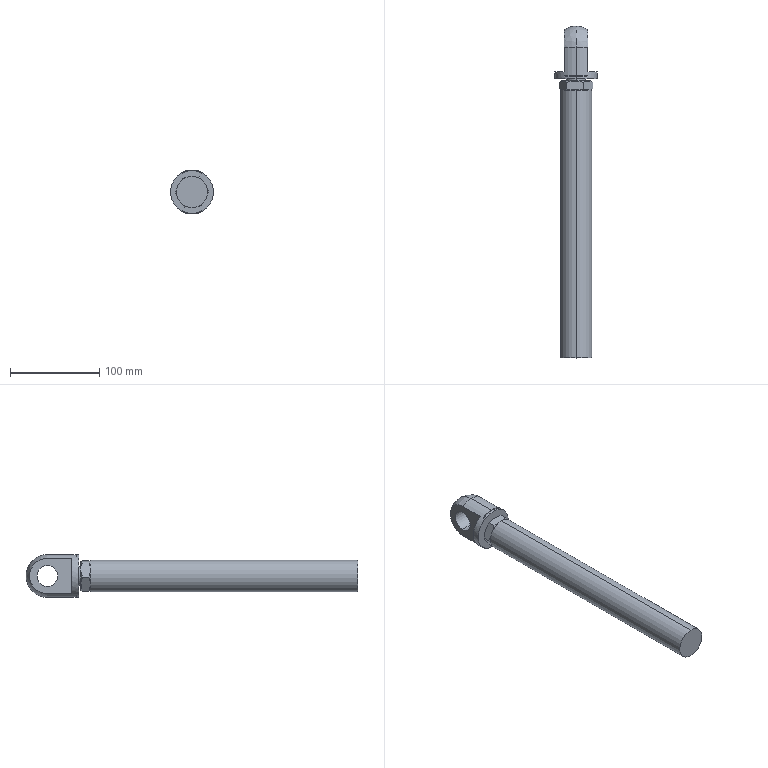Part | STEP file | Cylinder 2 | 3 solids | 46 faces | box 48 x 372 x 48.4 mm | volume 366109 mm3 | plane 22 | cylinder 14 | cone 8 | sphere 2 | commonest cylinder face diameters 20 x4 18.565 x2 21 x2 23.25 x2 35 x2 48 x2
STEP:
#1=CARTESIAN_POINT('',(-41.985,211.295,470.877));
#2=VERTEX_POINT('',#1);
#3=CARTESIAN_POINT('',(-40.938,211.901,470.948));
#4=VERTEX_POINT('',#3);
#5=CARTESIAN_POINT('',(-41.985,211.295,470.877));
#6=DIRECTION('',(0.864,0.5,0.05849));
#7=VECTOR('',#6,1000.);
#8=LINE('',#5,#7);
#9=EDGE_CURVE('',#2,#4,#8,.T.);
#10=ORIENTED_EDGE('',*,*,#9,.F.);
#11=CARTESIAN_POINT('',(-60.507,211.295,469.623));
#12=VERTEX_POINT('',#11);
#13=CARTESIAN_POINT('',(-51.246,211.295,470.25));
#14=DIRECTION('',(0.,1.,0.));
#15=DIRECTION('',(-0.9977,0.,-0.06754));
#16=AXIS2_PLACEMENT_3D('',#13,#14,#15);
#17=CIRCLE('',#16,9.282);
#18=EDGE_CURVE('',#12,#2,#17,.T.);
#19=ORIENTED_EDGE('',*,*,#18,.F.);
#20=CARTESIAN_POINT('',(-61.555,211.901,469.552));
#21=VERTEX_POINT('',#20);
#22=CARTESIAN_POINT('',(-60.507,211.295,469.623));
#23=DIRECTION('',(-0.864,0.5,-0.05849));
#24=VECTOR('',#23,1000.);
#25=LINE('',#22,#24);
#26=EDGE_CURVE('',#12,#21,#25,.T.);
#27=ORIENTED_EDGE('',*,*,#26,.T.);
#28=CARTESIAN_POINT('',(-51.246,211.901,470.25));
#29=DIRECTION('',(0.,-1.,0.));
#30=DIRECTION('',(-0.9977,0.,-0.06754));
#31=AXIS2_PLACEMENT_3D('',#28,#29,#30);
#32=CIRCLE('',#31,10.332);
#33=EDGE_CURVE('',#4,#21,#32,.T.);
#34=ORIENTED_EDGE('',*,*,#33,.F.);
#35=EDGE_LOOP('',(#10,#19,#27,#34));
#36=FACE_OUTER_BOUND('',#35,.T.);
#37=CARTESIAN_POINT('',(-51.246,211.295,470.25));
#38=DIRECTION('',(0.,1.,0.));
#39=DIRECTION('',(-0.9977,0.,-0.06754));
#40=AXIS2_PLACEMENT_3D('',#37,#38,#39);
#41=CONICAL_SURFACE('',#40,9.282,1.047);
#42=ADVANCED_FACE('',(#36),#41,.F.);
#43=CARTESIAN_POINT('',(-60.507,202.451,469.623));
#44=VERTEX_POINT('',#43);
#45=CARTESIAN_POINT('',(-61.112,201.401,469.582));
#46=VERTEX_POINT('',#45);
#47=CARTESIAN_POINT('',(-61.112,201.401,469.582));
#48=DIRECTION('',(-0.4989,-0.866,-0.03377));
#49=VECTOR('',#48,1000.);
#50=LINE('',#47,#49);
#51=EDGE_CURVE('',#44,#46,#50,.T.);
#52=ORIENTED_EDGE('',*,*,#51,.F.);
#53=CARTESIAN_POINT('',(-41.985,202.451,470.877));
#54=VERTEX_POINT('',#53);
#55=CARTESIAN_POINT('',(-51.246,202.451,470.25));
#56=DIRECTION('',(0.,-1.,0.));
#57=DIRECTION('',(-0.9977,0.,-0.06754));
#58=AXIS2_PLACEMENT_3D('',#55,#56,#57);
#59=CIRCLE('',#58,9.282);
#60=EDGE_CURVE('',#54,#44,#59,.T.);
#61=ORIENTED_EDGE('',*,*,#60,.F.);
#62=CARTESIAN_POINT('',(-41.381,201.401,470.918));
#63=VERTEX_POINT('',#62);
#64=CARTESIAN_POINT('',(-41.381,201.401,470.918));
#65=DIRECTION('',(0.4989,-0.866,0.03377));
#66=VECTOR('',#65,1000.);
#67=LINE('',#64,#66);
#68=EDGE_CURVE('',#54,#63,#67,.T.);
#69=ORIENTED_EDGE('',*,*,#68,.T.);
#70=CARTESIAN_POINT('',(-51.246,201.401,470.25));
#71=DIRECTION('',(0.,1.,0.));
#72=DIRECTION('',(-0.9977,0.,-0.06754));
#73=AXIS2_PLACEMENT_3D('',#70,#71,#72);
#74=CIRCLE('',#73,9.888);
#75=EDGE_CURVE('',#46,#63,#74,.T.);
#76=ORIENTED_EDGE('',*,*,#75,.F.);
#77=EDGE_LOOP('',(#52,#61,#69,#76));
#78=FACE_OUTER_BOUND('',#77,.T.);
#79=CARTESIAN_POINT('',(-51.246,201.401,470.25));
#80=DIRECTION('',(0.,-1.,0.));
#81=DIRECTION('',(0.9977,0.,0.06754));
#82=AXIS2_PLACEMENT_3D('',#79,#80,#81);
#83=CONICAL_SURFACE('',#82,9.888,0.5236);
#84=ADVANCED_FACE('',(#78),#83,.F.);
#85=CARTESIAN_POINT('',(-67.272,211.901,469.165));
#86=VERTEX_POINT('',#85);
#87=CARTESIAN_POINT('',(-69.967,210.341,468.983));
#88=VERTEX_POINT('',#87);
#89=CARTESIAN_POINT('',(-67.272,211.901,469.165));
#90=DIRECTION('',(-0.864,-0.5,-0.05849));
#91=VECTOR('',#90,1000.);
#92=LINE('',#89,#91);
#93=EDGE_CURVE('',#86,#88,#92,.T.);
#94=ORIENTED_EDGE('',*,*,#93,.F.);
#95=CARTESIAN_POINT('',(-35.221,211.901,471.335));
#96=VERTEX_POINT('',#95);
#97=CARTESIAN_POINT('',(-51.246,211.901,470.25));
#98=DIRECTION('',(0.,-1.,0.));
#99=DIRECTION('',(0.9977,0.,0.06754));
#100=AXIS2_PLACEMENT_3D('',#97,#98,#99);
#101=CIRCLE('',#100,16.063);
#102=EDGE_CURVE('',#86,#96,#101,.T.);
#103=ORIENTED_EDGE('',*,*,#102,.T.);
#104=CARTESIAN_POINT('',(-32.525,210.341,471.517));
#105=VERTEX_POINT('',#104);
#106=CARTESIAN_POINT('',(-35.221,211.901,471.335));
#107=DIRECTION('',(0.864,-0.5,0.05849));
#108=VECTOR('',#107,1000.);
#109=LINE('',#106,#108);
#110=EDGE_CURVE('',#96,#105,#109,.T.);
#111=ORIENTED_EDGE('',*,*,#110,.T.);
#112=CARTESIAN_POINT('',(-40.788,210.341,454.671));
#113=VERTEX_POINT('',#112);
#114=CARTESIAN_POINT('',(-32.525,210.341,471.517));
#115=CARTESIAN_POINT('',(-33.2,210.784,470.142));
#116=CARTESIAN_POINT('',(-33.879,211.148,468.757));
#117=CARTESIAN_POINT('',(-35.253,211.653,465.957));
#118=CARTESIAN_POINT('',(-35.946,211.792,464.542));
#119=CARTESIAN_POINT('',(-37.,211.793,462.394));
#120=CARTESIAN_POINT('',(-37.353,211.759,461.675));
#121=CARTESIAN_POINT('',(-38.051,211.627,460.251));
#122=CARTESIAN_POINT('',(-38.398,211.529,459.544));
#123=CARTESIAN_POINT('',(-39.432,211.15,457.436));
#124=CARTESIAN_POINT('',(-40.113,210.784,456.048));
#125=CARTESIAN_POINT('',(-40.788,210.341,454.671));
#126=B_SPLINE_CURVE_WITH_KNOTS('',3,(#114,#115,#116,#117,#118,#119,#120,#121,#122,#123,#124,#125),.UNSPECIFIED.,.F.,.F.,(4,2,2,2,2,4),(0.,0.004738,0.009475,0.01184,0.01421,0.01895),.UNSPECIFIED.);
#127=EDGE_CURVE('',#105,#113,#126,.T.);
#128=ORIENTED_EDGE('',*,*,#127,.T.);
#129=CARTESIAN_POINT('',(-59.509,210.341,453.403));
#130=VERTEX_POINT('',#129);
#131=CARTESIAN_POINT('',(-40.788,210.341,454.671));
#132=CARTESIAN_POINT('',(-42.317,210.784,454.567));
#133=CARTESIAN_POINT('',(-43.856,211.148,454.463));
#134=CARTESIAN_POINT('',(-46.967,211.653,454.252));
#135=CARTESIAN_POINT('',(-48.539,211.792,454.146));
#136=CARTESIAN_POINT('',(-50.927,211.793,453.984));
#137=CARTESIAN_POINT('',(-51.726,211.759,453.93));
#138=CARTESIAN_POINT('',(-53.308,211.627,453.823));
#139=CARTESIAN_POINT('',(-54.093,211.529,453.77));
#140=CARTESIAN_POINT('',(-56.436,211.15,453.612));
#141=CARTESIAN_POINT('',(-57.979,210.784,453.507));
#142=CARTESIAN_POINT('',(-59.509,210.341,453.403));
#143=B_SPLINE_CURVE_WITH_KNOTS('',3,(#131,#132,#133,#134,#135,#136,#137,#138,#139,#140,#141,#142),.UNSPECIFIED.,.F.,.F.,(4,2,2,2,2,4),(0.,0.004738,0.009475,0.01184,0.01421,0.01895),.UNSPECIFIED.);
#144=EDGE_CURVE('',#113,#130,#143,.T.);
#145=ORIENTED_EDGE('',*,*,#144,.T.);
#146=CARTESIAN_POINT('',(-59.509,210.341,453.403));
#147=CARTESIAN_POINT('',(-60.363,210.784,454.675));
#148=CARTESIAN_POINT('',(-61.223,211.148,455.957));
#149=CARTESIAN_POINT('',(-62.961,211.653,458.546));
#150=CARTESIAN_POINT('',(-63.839,211.792,459.854));
#151=CARTESIAN_POINT('',(-65.173,211.793,461.84));
#152=CARTESIAN_POINT('',(-65.62,211.759,462.506));
#153=CARTESIAN_POINT('',(-66.503,211.627,463.822));
#154=CARTESIAN_POINT('',(-66.942,211.529,464.476));
#155=CARTESIAN_POINT('',(-68.251,211.15,466.425));
#156=CARTESIAN_POINT('',(-69.113,210.784,467.709));
#157=CARTESIAN_POINT('',(-69.967,210.341,468.983));
#158=B_SPLINE_CURVE_WITH_KNOTS('',3,(#146,#147,#148,#149,#150,#151,#152,#153,#154,#155,#156,#157),.UNSPECIFIED.,.F.,.F.,(4,2,2,2,2,4),(0.,0.004738,0.009475,0.01184,0.01421,0.01895),.UNSPECIFIED.);
#159=EDGE_CURVE('',#130,#88,#158,.T.);
#160=ORIENTED_EDGE('',*,*,#159,.T.);
#161=EDGE_LOOP('',(#94,#103,#111,#128,#145,#160));
#162=FACE_OUTER_BOUND('',#161,.T.);
#163=CARTESIAN_POINT('',(-51.246,211.901,470.25));
#164=DIRECTION('',(0.,-1.,0.));
#165=DIRECTION('',(0.9977,0.,0.06754));
#166=AXIS2_PLACEMENT_3D('',#163,#164,#165);
#167=CONICAL_SURFACE('',#166,16.063,1.047);
#168=ADVANCED_FACE('',(#162),#167,.T.);
#169=CARTESIAN_POINT('',(-35.221,201.401,471.335));
#170=VERTEX_POINT('',#169);
#171=CARTESIAN_POINT('',(-32.525,202.961,471.517));
#172=VERTEX_POINT('',#171);
#173=CARTESIAN_POINT('',(-32.525,202.961,471.517));
#174=DIRECTION('',(0.864,0.5,0.05849));
#175=VECTOR('',#174,1000.);
#176=LINE('',#173,#175);
#177=EDGE_CURVE('',#170,#172,#176,.T.);
#178=ORIENTED_EDGE('',*,*,#177,.F.);
#179=CARTESIAN_POINT('',(-67.272,201.401,469.165));
#180=VERTEX_POINT('',#179);
#181=CARTESIAN_POINT('',(-51.246,201.401,470.25));
#182=DIRECTION('',(0.,-1.,0.));
#183=DIRECTION('',(0.9977,0.,0.06754));
#184=AXIS2_PLACEMENT_3D('',#181,#182,#183);
#185=CIRCLE('',#184,16.063);
#186=EDGE_CURVE('',#180,#170,#185,.T.);
#187=ORIENTED_EDGE('',*,*,#186,.F.);
#188=CARTESIAN_POINT('',(-69.967,202.961,468.983));
#189=VERTEX_POINT('',#188);
#190=CARTESIAN_POINT('',(-69.967,202.961,468.983));
#191=DIRECTION('',(-0.864,0.5,-0.05849));
#192=VECTOR('',#191,1000.);
#193=LINE('',#190,#192);
#194=EDGE_CURVE('',#180,#189,#193,.T.);
#195=ORIENTED_EDGE('',*,*,#194,.T.);
#196=CARTESIAN_POINT('',(-59.509,202.961,453.403));
#197=VERTEX_POINT('',#196);
#198=CARTESIAN_POINT('',(-69.967,202.961,468.983));
#199=CARTESIAN_POINT('',(-69.114,202.518,467.711));
#200=CARTESIAN_POINT('',(-68.254,202.154,466.43));
#201=CARTESIAN_POINT('',(-66.516,201.649,463.841));
#202=CARTESIAN_POINT('',(-65.638,201.51,462.532));
#203=CARTESIAN_POINT('',(-64.304,201.509,460.546));
#204=CARTESIAN_POINT('',(-63.857,201.543,459.88));
#205=CARTESIAN_POINT('',(-62.974,201.675,458.564));
#206=CARTESIAN_POINT('',(-62.535,201.773,457.91));
#207=CARTESIAN_POINT('',(-61.226,202.153,455.961));
#208=CARTESIAN_POINT('',(-60.364,202.518,454.677));
#209=CARTESIAN_POINT('',(-59.509,202.961,453.403));
#210=B_SPLINE_CURVE_WITH_KNOTS('',3,(#198,#199,#200,#201,#202,#203,#204,#205,#206,#207,#208,#209),.UNSPECIFIED.,.F.,.F.,(4,2,2,2,2,4),(0.,0.004738,0.009475,0.01184,0.01421,0.01895),.UNSPECIFIED.);
#211=EDGE_CURVE('',#189,#197,#210,.T.);
#212=ORIENTED_EDGE('',*,*,#211,.T.);
#213=CARTESIAN_POINT('',(-40.788,202.961,454.671));
#214=VERTEX_POINT('',#213);
#215=CARTESIAN_POINT('',(-59.509,202.961,453.403));
#216=CARTESIAN_POINT('',(-57.981,202.518,453.507));
#217=CARTESIAN_POINT('',(-56.441,202.154,453.611));
#218=CARTESIAN_POINT('',(-53.33,201.649,453.822));
#219=CARTESIAN_POINT('',(-51.758,201.51,453.928));
#220=CARTESIAN_POINT('',(-49.371,201.509,454.09));
#221=CARTESIAN_POINT('',(-48.571,201.543,454.144));
#222=CARTESIAN_POINT('',(-46.99,201.675,454.251));
#223=CARTESIAN_POINT('',(-46.204,201.773,454.304));
#224=CARTESIAN_POINT('',(-43.862,202.153,454.463));
#225=CARTESIAN_POINT('',(-42.319,202.518,454.567));
#226=CARTESIAN_POINT('',(-40.788,202.961,454.671));
#227=B_SPLINE_CURVE_WITH_KNOTS('',3,(#215,#216,#217,#218,#219,#220,#221,#222,#223,#224,#225,#226),.UNSPECIFIED.,.F.,.F.,(4,2,2,2,2,4),(0.,0.004738,0.009475,0.01184,0.01421,0.01895),.UNSPECIFIED.);
#228=EDGE_CURVE('',#197,#214,#227,.T.);
#229=ORIENTED_EDGE('',*,*,#228,.T.);
#230=CARTESIAN_POINT('',(-40.788,202.961,454.671));
#231=CARTESIAN_POINT('',(-40.114,202.518,456.046));
#232=CARTESIAN_POINT('',(-39.434,202.154,457.432));
#233=CARTESIAN_POINT('',(-38.061,201.649,460.231));
#234=CARTESIAN_POINT('',(-37.367,201.51,461.646));
#235=CARTESIAN_POINT('',(-36.314,201.509,463.794));
#236=CARTESIAN_POINT('',(-35.961,201.543,464.514));
#237=CARTESIAN_POINT('',(-35.263,201.675,465.937));
#238=CARTESIAN_POINT('',(-34.916,201.773,466.644));
#239=CARTESIAN_POINT('',(-33.882,202.153,468.752));
#240=CARTESIAN_POINT('',(-33.201,202.518,470.14));
#241=CARTESIAN_POINT('',(-32.525,202.961,471.517));
#242=B_SPLINE_CURVE_WITH_KNOTS('',3,(#230,#231,#232,#233,#234,#235,#236,#237,#238,#239,#240,#241),.UNSPECIFIED.,.F.,.F.,(4,2,2,2,2,4),(0.,0.004738,0.009475,0.01184,0.01421,0.01895),.UNSPECIFIED.);
#243=EDGE_CURVE('',#214,#172,#242,.T.);
#244=ORIENTED_EDGE('',*,*,#243,.T.);
#245=EDGE_LOOP('',(#178,#187,#195,#212,#229,#244));
#246=FACE_OUTER_BOUND('',#245,.T.);
#247=CARTESIAN_POINT('',(-51.246,202.961,470.25));
#248=DIRECTION('',(0.,1.,0.));
#249=DIRECTION('',(-0.9977,0.,-0.06754));
#250=AXIS2_PLACEMENT_3D('',#247,#248,#249);
#251=CONICAL_SURFACE('',#250,18.764,1.047);
#252=ADVANCED_FACE('',(#246),#251,.T.);
#253=CARTESIAN_POINT('',(-41.985,201.401,470.877));
#254=DIRECTION('',(0.,1.,0.));
#255=VECTOR('',#254,1000.);
#256=LINE('',#253,#255);
#257=EDGE_CURVE('',#54,#2,#256,.T.);
#258=ORIENTED_EDGE('',*,*,#257,.F.);
#259=ORIENTED_EDGE('',*,*,#60,.T.);
#260=CARTESIAN_POINT('',(-60.507,201.401,469.623));
#261=DIRECTION('',(0.,1.,0.));
#262=VECTOR('',#261,1000.);
#263=LINE('',#260,#262);
#264=EDGE_CURVE('',#44,#12,#263,.T.);
#265=ORIENTED_EDGE('',*,*,#264,.T.);
#266=ORIENTED_EDGE('',*,*,#18,.T.);
#267=EDGE_LOOP('',(#258,#259,#265,#266));
#268=FACE_OUTER_BOUND('',#267,.T.);
#269=CARTESIAN_POINT('',(-51.246,201.401,470.25));
#270=DIRECTION('',(0.,1.,0.));
#271=DIRECTION('',(-0.9977,0.,-0.06754));
#272=AXIS2_PLACEMENT_3D('',#269,#270,#271);
#273=CYLINDRICAL_SURFACE('',#272,9.282);
#274=ADVANCED_FACE('',(#268),#273,.F.);
#275=CARTESIAN_POINT('',(-51.246,211.901,470.25));
#276=DIRECTION('',(0.,-1.,0.));
#277=DIRECTION('',(-0.9977,0.,-0.06754));
#278=AXIS2_PLACEMENT_3D('',#275,#276,#277);
#279=CIRCLE('',#278,10.332);
#280=EDGE_CURVE('',#21,#4,#279,.T.);
#281=ORIENTED_EDGE('',*,*,#280,.T.);
#282=ORIENTED_EDGE('',*,*,#33,.T.);
#283=EDGE_LOOP('',(#281,#282));
#284=FACE_BOUND('',#283,.T.);
#285=CARTESIAN_POINT('',(-51.246,211.901,470.25));
#286=DIRECTION('',(0.,-1.,0.));
#287=DIRECTION('',(0.9977,0.,0.06754));
#288=AXIS2_PLACEMENT_3D('',#285,#286,#287);
#289=CIRCLE('',#288,16.063);
#290=EDGE_CURVE('',#96,#86,#289,.T.);
#291=ORIENTED_EDGE('',*,*,#290,.F.);
#292=ORIENTED_EDGE('',*,*,#102,.F.);
#293=EDGE_LOOP('',(#291,#292));
#294=FACE_OUTER_BOUND('',#293,.T.);
#295=CARTESIAN_POINT('',(-59.509,211.901,453.403));
#296=DIRECTION('',(0.,1.,0.));
#297=DIRECTION('',(-0.9977,0.,-0.06754));
#298=AXIS2_PLACEMENT_3D('',#295,#296,#297);
#299=PLANE('',#298);
#300=ADVANCED_FACE('',(#284,#294),#299,.T.);
#301=CARTESIAN_POINT('',(-51.246,201.401,470.25));
#302=DIRECTION('',(0.,1.,0.));
#303=DIRECTION('',(-0.9977,0.,-0.06754));
#304=AXIS2_PLACEMENT_3D('',#301,#302,#303);
#305=CIRCLE('',#304,9.888);
#306=EDGE_CURVE('',#63,#46,#305,.T.);
#307=ORIENTED_EDGE('',*,*,#306,.T.);
#308=ORIENTED_EDGE('',*,*,#75,.T.);
#309=EDGE_LOOP('',(#307,#308));
#310=FACE_BOUND('',#309,.T.);
#311=ORIENTED_EDGE('',*,*,#186,.T.);
#312=CARTESIAN_POINT('',(-51.246,201.401,470.25));
#313=DIRECTION('',(0.,-1.,0.));
#314=DIRECTION('',(0.9977,0.,0.06754));
#315=AXIS2_PLACEMENT_3D('',#312,#313,#314);
#316=CIRCLE('',#315,16.063);
#317=EDGE_CURVE('',#170,#180,#316,.T.);
#318=ORIENTED_EDGE('',*,*,#317,.T.);
#319=EDGE_LOOP('',(#311,#318));
#320=FACE_OUTER_BOUND('',#319,.T.);
#321=CARTESIAN_POINT('',(-59.509,201.401,453.403));
#322=DIRECTION('',(0.,1.,0.));
#323=DIRECTION('',(-0.9977,0.,-0.06754));
#324=AXIS2_PLACEMENT_3D('',#321,#322,#323);
#325=PLANE('',#324);
#326=ADVANCED_FACE('',(#310,#320),#325,.F.);
#327=ORIENTED_EDGE('',*,*,#159,.F.);
#328=CARTESIAN_POINT('',(-59.509,201.401,453.403));
#329=DIRECTION('',(0.,1.,0.));
#330=VECTOR('',#329,1000.);
#331=LINE('',#328,#330);
#332=EDGE_CURVE('',#197,#130,#331,.T.);
#333=ORIENTED_EDGE('',*,*,#332,.F.);
#334=ORIENTED_EDGE('',*,*,#211,.F.);
#335=CARTESIAN_POINT('',(-69.967,201.401,468.983));
#336=DIRECTION('',(0.,1.,0.));
#337=VECTOR('',#336,1000.);
#338=LINE('',#335,#337);
#339=EDGE_CURVE('',#189,#88,#338,.T.);
#340=ORIENTED_EDGE('',*,*,#339,.T.);
#341=EDGE_LOOP('',(#327,#333,#334,#340));
#342=FACE_OUTER_BOUND('',#341,.T.);
#343=CARTESIAN_POINT('',(-59.509,201.401,453.403));
#344=DIRECTION('',(-0.8303,0.,-0.5573));
#345=DIRECTION('',(0.,-1.,0.));
#346=AXIS2_PLACEMENT_3D('',#343,#344,#345);
#347=PLANE('',#346);
#348=ADVANCED_FACE('',(#342),#347,.T.);
#349=CARTESIAN_POINT('',(-61.704,210.341,485.829));
#350=VERTEX_POINT('',#349);
#351=CARTESIAN_POINT('',(-69.967,210.341,468.983));
#352=CARTESIAN_POINT('',(-69.293,210.784,470.358));
#353=CARTESIAN_POINT('',(-68.613,211.148,471.743));
#354=CARTESIAN_POINT('',(-67.24,211.653,474.543));
#355=CARTESIAN_POINT('',(-66.546,211.792,475.958));
#356=CARTESIAN_POINT('',(-65.493,211.793,478.106));
#357=CARTESIAN_POINT('',(-65.14,211.759,478.825));
#358=CARTESIAN_POINT('',(-64.442,211.627,480.249));
#359=CARTESIAN_POINT('',(-64.095,211.529,480.956));
#360=CARTESIAN_POINT('',(-63.061,211.15,483.064));
#361=CARTESIAN_POINT('',(-62.38,210.784,484.452));
#362=CARTESIAN_POINT('',(-61.704,210.341,485.829));
#363=B_SPLINE_CURVE_WITH_KNOTS('',3,(#351,#352,#353,#354,#355,#356,#357,#358,#359,#360,#361,#362),.UNSPECIFIED.,.F.,.F.,(4,2,2,2,2,4),(0.,0.004738,0.009475,0.01184,0.01421,0.01895),.UNSPECIFIED.);
#364=EDGE_CURVE('',#88,#350,#363,.T.);
#365=ORIENTED_EDGE('',*,*,#364,.F.);
#366=ORIENTED_EDGE('',*,*,#339,.F.);
#367=CARTESIAN_POINT('',(-61.704,202.961,485.829));
#368=VERTEX_POINT('',#367);
#369=CARTESIAN_POINT('',(-61.704,202.961,485.829));
#370=CARTESIAN_POINT('',(-62.379,202.518,484.454));
#371=CARTESIAN_POINT('',(-63.059,202.154,483.068));
#372=CARTESIAN_POINT('',(-64.432,201.649,480.269));
#373=CARTESIAN_POINT('',(-65.126,201.51,478.854));
#374=CARTESIAN_POINT('',(-66.179,201.509,476.706));
#375=CARTESIAN_POINT('',(-66.532,201.543,475.986));
#376=CARTESIAN_POINT('',(-67.23,201.675,474.563));
#377=CARTESIAN_POINT('',(-67.577,201.773,473.856));
#378=CARTESIAN_POINT('',(-68.611,202.153,471.748));
#379=CARTESIAN_POINT('',(-69.292,202.518,470.36));
#380=CARTESIAN_POINT('',(-69.967,202.961,468.983));
#381=B_SPLINE_CURVE_WITH_KNOTS('',3,(#369,#370,#371,#372,#373,#374,#375,#376,#377,#378,#379,#380),.UNSPECIFIED.,.F.,.F.,(4,2,2,2,2,4),(0.,0.004738,0.009475,0.01184,0.01421,0.01895),.UNSPECIFIED.);
#382=EDGE_CURVE('',#368,#189,#381,.T.);
#383=ORIENTED_EDGE('',*,*,#382,.F.);
#384=CARTESIAN_POINT('',(-61.704,201.401,485.829));
#385=DIRECTION('',(0.,1.,0.));
#386=VECTOR('',#385,1000.);
#387=LINE('',#384,#386);
#388=EDGE_CURVE('',#368,#350,#387,.T.);
#389=ORIENTED_EDGE('',*,*,#388,.T.);
#390=EDGE_LOOP('',(#365,#366,#383,#389));
#391=FACE_OUTER_BOUND('',#390,.T.);
#392=CARTESIAN_POINT('',(-69.967,201.401,468.983));
#393=DIRECTION('',(-0.8978,0.,0.4404));
#394=DIRECTION('',(0.,-1.,0.));
#395=AXIS2_PLACEMENT_3D('',#392,#393,#394);
#396=PLANE('',#395);
#397=ADVANCED_FACE('',(#391),#396,.T.);
#398=CARTESIAN_POINT('',(-42.983,210.341,487.097));
#399=VERTEX_POINT('',#398);
#400=CARTESIAN_POINT('',(-61.704,210.341,485.829));
#401=CARTESIAN_POINT('',(-60.176,210.784,485.933));
#402=CARTESIAN_POINT('',(-58.637,211.148,486.037));
#403=CARTESIAN_POINT('',(-55.525,211.653,486.248));
#404=CARTESIAN_POINT('',(-53.953,211.792,486.354));
#405=CARTESIAN_POINT('',(-51.566,211.793,486.516));
#406=CARTESIAN_POINT('',(-50.766,211.759,486.57));
#407=CARTESIAN_POINT('',(-49.185,211.627,486.677));
#408=CARTESIAN_POINT('',(-48.399,211.529,486.73));
#409=CARTESIAN_POINT('',(-46.057,211.15,486.888));
#410=CARTESIAN_POINT('',(-44.514,210.784,486.993));
#411=CARTESIAN_POINT('',(-42.983,210.341,487.097));
#412=B_SPLINE_CURVE_WITH_KNOTS('',3,(#400,#401,#402,#403,#404,#405,#406,#407,#408,#409,#410,#411),.UNSPECIFIED.,.F.,.F.,(4,2,2,2,2,4),(0.,0.004738,0.009475,0.01184,0.01421,0.01895),.UNSPECIFIED.);
#413=EDGE_CURVE('',#350,#399,#412,.T.);
#414=ORIENTED_EDGE('',*,*,#413,.F.);
#415=ORIENTED_EDGE('',*,*,#388,.F.);
#416=CARTESIAN_POINT('',(-42.983,202.961,487.097));
#417=VERTEX_POINT('',#416);
#418=CARTESIAN_POINT('',(-42.983,202.961,487.097));
#419=CARTESIAN_POINT('',(-44.512,202.518,486.993));
#420=CARTESIAN_POINT('',(-46.051,202.154,486.889));
#421=CARTESIAN_POINT('',(-49.163,201.649,486.678));
#422=CARTESIAN_POINT('',(-50.734,201.51,486.572));
#423=CARTESIAN_POINT('',(-53.122,201.509,486.41));
#424=CARTESIAN_POINT('',(-53.921,201.543,486.356));
#425=CARTESIAN_POINT('',(-55.503,201.675,486.249));
#426=CARTESIAN_POINT('',(-56.289,201.773,486.196));
#427=CARTESIAN_POINT('',(-58.631,202.153,486.037));
#428=CARTESIAN_POINT('',(-60.174,202.518,485.933));
#429=CARTESIAN_POINT('',(-61.704,202.961,485.829));
#430=B_SPLINE_CURVE_WITH_KNOTS('',3,(#418,#419,#420,#421,#422,#423,#424,#425,#426,#427,#428,#429),.UNSPECIFIED.,.F.,.F.,(4,2,2,2,2,4),(0.,0.004738,0.009475,0.01184,0.01421,0.01895),.UNSPECIFIED.);
#431=EDGE_CURVE('',#417,#368,#430,.T.);
#432=ORIENTED_EDGE('',*,*,#431,.F.);
#433=CARTESIAN_POINT('',(-42.983,201.401,487.097));
#434=DIRECTION('',(0.,1.,0.));
#435=VECTOR('',#434,1000.);
#436=LINE('',#433,#435);
#437=EDGE_CURVE('',#417,#399,#436,.T.);
#438=ORIENTED_EDGE('',*,*,#437,.T.);
#439=EDGE_LOOP('',(#414,#415,#432,#438));
#440=FACE_OUTER_BOUND('',#439,.T.);
#441=CARTESIAN_POINT('',(-61.704,201.401,485.829));
#442=DIRECTION('',(-0.06754,0.,0.9977));
#443=DIRECTION('',(-0.9977,0.,-0.06754));
#444=AXIS2_PLACEMENT_3D('',#441,#442,#443);
#445=PLANE('',#444);
#446=ADVANCED_FACE('',(#440),#445,.T.);
#447=CARTESIAN_POINT('',(-42.983,210.341,487.097));
#448=CARTESIAN_POINT('',(-42.13,210.784,485.825));
#449=CARTESIAN_POINT('',(-41.27,211.148,484.543));
#450=CARTESIAN_POINT('',(-39.532,211.653,481.954));
#451=CARTESIAN_POINT('',(-38.654,211.792,480.646));
#452=CARTESIAN_POINT('',(-37.32,211.793,478.66));
#453=CARTESIAN_POINT('',(-36.873,211.759,477.994));
#454=CARTESIAN_POINT('',(-35.99,211.627,476.678));
#455=CARTESIAN_POINT('',(-35.551,211.529,476.024));
#456=CARTESIAN_POINT('',(-34.242,211.15,474.075));
#457=CARTESIAN_POINT('',(-33.38,210.784,472.791));
#458=CARTESIAN_POINT('',(-32.525,210.341,471.517));
#459=B_SPLINE_CURVE_WITH_KNOTS('',3,(#447,#448,#449,#450,#451,#452,#453,#454,#455,#456,#457,#458),.UNSPECIFIED.,.F.,.F.,(4,2,2,2,2,4),(0.,0.004738,0.009475,0.01184,0.01421,0.01895),.UNSPECIFIED.);
#460=EDGE_CURVE('',#399,#105,#459,.T.);
#461=ORIENTED_EDGE('',*,*,#460,.F.);
#462=ORIENTED_EDGE('',*,*,#437,.F.);
#463=CARTESIAN_POINT('',(-32.525,202.961,471.517));
#464=CARTESIAN_POINT('',(-33.379,202.518,472.789));
#465=CARTESIAN_POINT('',(-34.239,202.154,474.07));
#466=CARTESIAN_POINT('',(-35.977,201.649,476.659));
#467=CARTESIAN_POINT('',(-36.855,201.51,477.968));
#468=CARTESIAN_POINT('',(-38.189,201.509,479.954));
#469=CARTESIAN_POINT('',(-38.636,201.543,480.62));
#470=CARTESIAN_POINT('',(-39.519,201.675,481.936));
#471=CARTESIAN_POINT('',(-39.958,201.773,482.59));
#472=CARTESIAN_POINT('',(-41.267,202.153,484.539));
#473=CARTESIAN_POINT('',(-42.129,202.518,485.823));
#474=CARTESIAN_POINT('',(-42.983,202.961,487.097));
#475=B_SPLINE_CURVE_WITH_KNOTS('',3,(#463,#464,#465,#466,#467,#468,#469,#470,#471,#472,#473,#474),.UNSPECIFIED.,.F.,.F.,(4,2,2,2,2,4),(0.,0.004738,0.009475,0.01184,0.01421,0.01895),.UNSPECIFIED.);
#476=EDGE_CURVE('',#172,#417,#475,.T.);
#477=ORIENTED_EDGE('',*,*,#476,.F.);
#478=CARTESIAN_POINT('',(-32.525,201.401,471.517));
#479=DIRECTION('',(0.,1.,0.));
#480=VECTOR('',#479,1000.);
#481=LINE('',#478,#480);
#482=EDGE_CURVE('',#172,#105,#481,.T.);
#483=ORIENTED_EDGE('',*,*,#482,.T.);
#484=EDGE_LOOP('',(#461,#462,#477,#483));
#485=FACE_OUTER_BOUND('',#484,.T.);
#486=CARTESIAN_POINT('',(-42.983,201.401,487.097));
#487=DIRECTION('',(0.8303,0.,0.5573));
#488=DIRECTION('',(0.,1.,0.));
#489=AXIS2_PLACEMENT_3D('',#486,#487,#488);
#490=PLANE('',#489);
#491=ADVANCED_FACE('',(#485),#490,.T.);
#492=ORIENTED_EDGE('',*,*,#127,.F.);
#493=ORIENTED_EDGE('',*,*,#482,.F.);
#494=ORIENTED_EDGE('',*,*,#243,.F.);
#495=CARTESIAN_POINT('',(-40.788,201.401,454.671));
#496=DIRECTION('',(0.,1.,0.));
#497=VECTOR('',#496,1000.);
#498=LINE('',#495,#497);
#499=EDGE_CURVE('',#214,#113,#498,.T.);
#500=ORIENTED_EDGE('',*,*,#499,.T.);
#501=EDGE_LOOP('',(#492,#493,#494,#500));
#502=FACE_OUTER_BOUND('',#501,.T.);
#503=CARTESIAN_POINT('',(-32.525,201.401,471.517));
#504=DIRECTION('',(0.8978,0.,-0.4404));
#505=DIRECTION('',(0.4404,0.,0.8978));
#506=AXIS2_PLACEMENT_3D('',#503,#504,#505);
#507=PLANE('',#506);
#508=ADVANCED_FACE('',(#502),#507,.T.);
#509=ORIENTED_EDGE('',*,*,#144,.F.);
#510=ORIENTED_EDGE('',*,*,#499,.F.);
#511=ORIENTED_EDGE('',*,*,#228,.F.);
#512=ORIENTED_EDGE('',*,*,#332,.T.);
#513=EDGE_LOOP('',(#509,#510,#511,#512));
#514=FACE_OUTER_BOUND('',#513,.T.);
#515=CARTESIAN_POINT('',(-40.788,201.401,454.671));
#516=DIRECTION('',(0.06754,0.,-0.9977));
#517=DIRECTION('',(0.,-1.,0.));
#518=AXIS2_PLACEMENT_3D('',#515,#516,#517);
#519=PLANE('',#518);
#520=ADVANCED_FACE('',(#514),#519,.T.);
#521=CARTESIAN_POINT('',(-51.246,202.451,470.25));
#522=DIRECTION('',(0.,-1.,0.));
#523=DIRECTION('',(-0.9977,0.,-0.06754));
#524=AXIS2_PLACEMENT_3D('',#521,#522,#523);
#525=CIRCLE('',#524,9.282);
#526=EDGE_CURVE('',#44,#54,#525,.T.);
#527=ORIENTED_EDGE('',*,*,#526,.T.);
#528=ORIENTED_EDGE('',*,*,#257,.T.);
#529=CARTESIAN_POINT('',(-51.246,211.295,470.25));
#530=DIRECTION('',(0.,1.,0.));
#531=DIRECTION('',(-0.9977,0.,-0.06754));
#532=AXIS2_PLACEMENT_3D('',#529,#530,#531);
#533=CIRCLE('',#532,9.282);
#534=EDGE_CURVE('',#2,#12,#533,.T.);
#535=ORIENTED_EDGE('',*,*,#534,.T.);
#536=ORIENTED_EDGE('',*,*,#264,.F.);
#537=EDGE_LOOP('',(#527,#528,#535,#536));
#538=FACE_OUTER_BOUND('',#537,.T.);
#539=CARTESIAN_POINT('',(-51.246,201.401,470.25));
#540=DIRECTION('',(0.,1.,0.));
#541=DIRECTION('',(-0.9977,0.,-0.06754));
#542=AXIS2_PLACEMENT_3D('',#539,#540,#541);
#543=CYLINDRICAL_SURFACE('',#542,9.282);
#544=ADVANCED_FACE('',(#538),#543,.F.);
#545=ORIENTED_EDGE('',*,*,#317,.F.);
#546=ORIENTED_EDGE('',*,*,#177,.T.);
#547=ORIENTED_EDGE('',*,*,#476,.T.);
#548=ORIENTED_EDGE('',*,*,#431,.T.);
#549=ORIENTED_EDGE('',*,*,#382,.T.);
#550=ORIENTED_EDGE('',*,*,#194,.F.);
#551=EDGE_LOOP('',(#545,#546,#547,#548,#549,#550));
#552=FACE_OUTER_BOUND('',#551,.T.);
#553=CARTESIAN_POINT('',(-51.246,202.961,470.25));
#554=DIRECTION('',(0.,1.,0.));
#555=DIRECTION('',(-0.9977,0.,-0.06754));
#556=AXIS2_PLACEMENT_3D('',#553,#554,#555);
#557=CONICAL_SURFACE('',#556,18.764,1.047);
#558=ADVANCED_FACE('',(#552),#557,.T.);
#559=ORIENTED_EDGE('',*,*,#290,.T.);
#560=ORIENTED_EDGE('',*,*,#93,.T.);
#561=ORIENTED_EDGE('',*,*,#364,.T.);
#562=ORIENTED_EDGE('',*,*,#413,.T.);
#563=ORIENTED_EDGE('',*,*,#460,.T.);
#564=ORIENTED_EDGE('',*,*,#110,.F.);
#565=EDGE_LOOP('',(#559,#560,#561,#562,#563,#564));
#566=FACE_OUTER_BOUND('',#565,.T.);
#567=CARTESIAN_POINT('',(-51.246,211.901,470.25));
#568=DIRECTION('',(0.,-1.,0.));
#569=DIRECTION('',(0.9977,0.,0.06754));
#570=AXIS2_PLACEMENT_3D('',#567,#568,#569);
#571=CONICAL_SURFACE('',#570,16.063,1.047);
#572=ADVANCED_FACE('',(#566),#571,.T.);
#573=ORIENTED_EDGE('',*,*,#526,.F.);
#574=ORIENTED_EDGE('',*,*,#51,.T.);
#575=ORIENTED_EDGE('',*,*,#306,.F.);
#576=ORIENTED_EDGE('',*,*,#68,.F.);
#577=EDGE_LOOP('',(#573,#574,#575,#576));
#578=FACE_OUTER_BOUND('',#577,.T.);
#579=CARTESIAN_POINT('',(-51.246,201.401,470.25));
#580=DIRECTION('',(0.,-1.,0.));
#581=DIRECTION('',(0.9977,0.,0.06754));
#582=AXIS2_PLACEMENT_3D('',#579,#580,#581);
#583=CONICAL_SURFACE('',#582,9.888,0.5236);
#584=ADVANCED_FACE('',(#578),#583,.F.);
#585=ORIENTED_EDGE('',*,*,#534,.F.);
#586=ORIENTED_EDGE('',*,*,#9,.T.);
#587=ORIENTED_EDGE('',*,*,#280,.F.);
#588=ORIENTED_EDGE('',*,*,#26,.F.);
#589=EDGE_LOOP('',(#585,#586,#587,#588));
#590=FACE_OUTER_BOUND('',#589,.T.);
#591=CARTESIAN_POINT('',(-51.246,211.295,470.25));
#592=DIRECTION('',(0.,1.,0.));
#593=DIRECTION('',(-0.9977,0.,-0.06754));
#594=AXIS2_PLACEMENT_3D('',#591,#592,#593);
#595=CONICAL_SURFACE('',#594,9.282,1.047);
#596=ADVANCED_FACE('',(#590),#595,.F.);
#597=CLOSED_SHELL('',(#42,#84,#168,#252,#274,#300,#326,#348,#397,#446,#491,#508,#520,#544,#558,#572,#584,#596));
#598=MANIFOLD_SOLID_BREP('',#597);
#599=CARTESIAN_POINT('',(-51.246,-98.599,452.75));
#600=VERTEX_POINT('',#599);
#601=CARTESIAN_POINT('',(-51.246,-98.599,487.75));
#602=VERTEX_POINT('',#601);
#603=CARTESIAN_POINT('',(-51.246,-98.599,470.25));
#604=DIRECTION('',(0.,1.,0.));
#605=DIRECTION('',(0.,0.,1.));
#606=AXIS2_PLACEMENT_3D('',#603,#604,#605);
#607=CIRCLE('',#606,17.5);
#608=EDGE_CURVE('',#600,#602,#607,.T.);
#609=ORIENTED_EDGE('',*,*,#608,.F.);
#610=CARTESIAN_POINT('',(-51.246,-98.599,470.25));
#611=DIRECTION('',(0.,1.,0.));
#612=DIRECTION('',(0.,0.,1.));
#613=AXIS2_PLACEMENT_3D('',#610,#611,#612);
#614=CIRCLE('',#613,17.5);
#615=EDGE_CURVE('',#602,#600,#614,.T.);
#616=ORIENTED_EDGE('',*,*,#615,.F.);
#617=EDGE_LOOP('',(#609,#616));
#618=FACE_OUTER_BOUND('',#617,.T.);
#619=CARTESIAN_POINT('',(-51.246,-98.599,470.25));
#620=DIRECTION('',(0.,1.,0.));
#621=DIRECTION('',(1.,0.,0.));
#622=AXIS2_PLACEMENT_3D('',#619,#620,#621);
#623=PLANE('',#622);
#624=ADVANCED_FACE('',(#618),#623,.F.);
#625=CARTESIAN_POINT('',(-51.246,201.401,452.75));
#626=VERTEX_POINT('',#625);
#627=CARTESIAN_POINT('',(-51.246,201.401,487.75));
#628=VERTEX_POINT('',#627);
#629=CARTESIAN_POINT('',(-51.246,201.401,470.25));
#630=DIRECTION('',(0.,1.,0.));
#631=DIRECTION('',(0.,0.,1.));
#632=AXIS2_PLACEMENT_3D('',#629,#630,#631);
#633=CIRCLE('',#632,17.5);
#634=EDGE_CURVE('',#626,#628,#633,.T.);
#635=ORIENTED_EDGE('',*,*,#634,.T.);
#636=CARTESIAN_POINT('',(-51.246,201.401,470.25));
#637=DIRECTION('',(0.,1.,0.));
#638=DIRECTION('',(0.,0.,1.));
#639=AXIS2_PLACEMENT_3D('',#636,#637,#638);
#640=CIRCLE('',#639,17.5);
#641=EDGE_CURVE('',#628,#626,#640,.T.);
#642=ORIENTED_EDGE('',*,*,#641,.T.);
#643=EDGE_LOOP('',(#635,#642));
#644=FACE_OUTER_BOUND('',#643,.T.);
#645=CARTESIAN_POINT('',(-51.246,201.401,470.25));
#646=DIRECTION('',(0.,1.,0.));
#647=DIRECTION('',(1.,0.,0.));
#648=AXIS2_PLACEMENT_3D('',#645,#646,#647);
#649=PLANE('',#648);
#650=ADVANCED_FACE('',(#644),#649,.T.);
#651=CARTESIAN_POINT('',(-51.246,201.401,487.75));
#652=DIRECTION('',(0.,-1.,0.));
#653=VECTOR('',#652,1000.);
#654=LINE('',#651,#653);
#655=EDGE_CURVE('',#628,#602,#654,.T.);
#656=ORIENTED_EDGE('',*,*,#655,.F.);
#657=ORIENTED_EDGE('',*,*,#634,.F.);
#658=CARTESIAN_POINT('',(-51.246,201.401,452.75));
#659=DIRECTION('',(0.,-1.,0.));
#660=VECTOR('',#659,1000.);
#661=LINE('',#658,#660);
#662=EDGE_CURVE('',#626,#600,#661,.T.);
#663=ORIENTED_EDGE('',*,*,#662,.T.);
#664=ORIENTED_EDGE('',*,*,#608,.T.);
#665=EDGE_LOOP('',(#656,#657,#663,#664));
#666=FACE_OUTER_BOUND('',#665,.T.);
#667=CARTESIAN_POINT('',(-51.246,201.401,470.25));
#668=DIRECTION('',(0.,-1.,0.));
#669=DIRECTION('',(0.,0.,-1.));
#670=AXIS2_PLACEMENT_3D('',#667,#668,#669);
#671=CYLINDRICAL_SURFACE('',#670,17.5);
#672=ADVANCED_FACE('',(#666),#671,.T.);
#673=ORIENTED_EDGE('',*,*,#641,.F.);
#674=ORIENTED_EDGE('',*,*,#655,.T.);
#675=ORIENTED_EDGE('',*,*,#615,.T.);
#676=ORIENTED_EDGE('',*,*,#662,.F.);
#677=EDGE_LOOP('',(#673,#674,#675,#676));
#678=FACE_OUTER_BOUND('',#677,.T.);
#679=CARTESIAN_POINT('',(-51.246,201.401,470.25));
#680=DIRECTION('',(0.,-1.,0.));
#681=DIRECTION('',(0.,0.,-1.));
#682=AXIS2_PLACEMENT_3D('',#679,#680,#681);
#683=CYLINDRICAL_SURFACE('',#682,17.5);
#684=ADVANCED_FACE('',(#678),#683,.T.);
#685=CLOSED_SHELL('',(#624,#650,#672,#684));
#686=MANIFOLD_SOLID_BREP('',#685);
#687=CARTESIAN_POINT('',(-64.496,217.354,490.261));
#688=VERTEX_POINT('',#687);
#689=CARTESIAN_POINT('',(-64.496,216.854,490.261));
#690=VERTEX_POINT('',#689);
#691=CARTESIAN_POINT('',(-64.496,214.401,490.261));
#692=DIRECTION('',(0.,-1.,0.));
#693=VECTOR('',#692,1000.);
#694=LINE('',#691,#693);
#695=EDGE_CURVE('',#688,#690,#694,.T.);
#696=ORIENTED_EDGE('',*,*,#695,.F.);
#697=CARTESIAN_POINT('',(-51.246,217.354,494.25));
#698=VERTEX_POINT('',#697);
#699=CARTESIAN_POINT('',(-51.246,217.354,470.25));
#700=DIRECTION('',(0.,1.,0.));
#701=DIRECTION('',(0.,0.,-1.));
#702=AXIS2_PLACEMENT_3D('',#699,#700,#701);
#703=CIRCLE('',#702,24.);
#704=EDGE_CURVE('',#688,#698,#703,.T.);
#705=ORIENTED_EDGE('',*,*,#704,.T.);
#706=CARTESIAN_POINT('',(-51.246,249.401,494.25));
#707=VERTEX_POINT('',#706);
#708=CARTESIAN_POINT('',(-51.246,214.401,494.25));
#709=DIRECTION('',(0.,1.,0.));
#710=VECTOR('',#709,1000.);
#711=LINE('',#708,#710);
#712=EDGE_CURVE('',#698,#707,#711,.T.);
#713=ORIENTED_EDGE('',*,*,#712,.T.);
#714=CARTESIAN_POINT('',(-64.496,249.401,490.261));
#715=VERTEX_POINT('',#714);
#716=CARTESIAN_POINT('',(-51.246,249.401,470.25));
#717=DIRECTION('',(0.,1.,0.));
#718=DIRECTION('',(0.,0.,1.));
#719=AXIS2_PLACEMENT_3D('',#716,#717,#718);
#720=CIRCLE('',#719,24.);
#721=EDGE_CURVE('',#715,#707,#720,.T.);
#722=ORIENTED_EDGE('',*,*,#721,.F.);
#723=CARTESIAN_POINT('',(-64.496,221.901,490.261));
#724=VERTEX_POINT('',#723);
#725=CARTESIAN_POINT('',(-64.496,273.401,490.261));
#726=DIRECTION('',(0.,-1.,0.));
#727=VECTOR('',#726,1000.);
#728=LINE('',#725,#727);
#729=EDGE_CURVE('',#715,#724,#728,.T.);
#730=ORIENTED_EDGE('',*,*,#729,.T.);
#731=CARTESIAN_POINT('',(-64.496,221.901,450.239));
#732=VERTEX_POINT('',#731);
#733=CARTESIAN_POINT('',(-51.246,221.901,470.25));
#734=DIRECTION('',(0.,-1.,0.));
#735=DIRECTION('',(0.,0.,-1.));
#736=AXIS2_PLACEMENT_3D('',#733,#734,#735);
#737=CIRCLE('',#736,24.);
#738=EDGE_CURVE('',#724,#732,#737,.T.);
#739=ORIENTED_EDGE('',*,*,#738,.T.);
#740=CARTESIAN_POINT('',(-64.496,249.401,450.239));
#741=VERTEX_POINT('',#740);
#742=CARTESIAN_POINT('',(-64.496,273.401,450.239));
#743=DIRECTION('',(0.,-1.,0.));
#744=VECTOR('',#743,1000.);
#745=LINE('',#742,#744);
#746=EDGE_CURVE('',#741,#732,#745,.T.);
#747=ORIENTED_EDGE('',*,*,#746,.F.);
#748=CARTESIAN_POINT('',(-51.246,249.401,446.25));
#749=VERTEX_POINT('',#748);
#750=CARTESIAN_POINT('',(-51.246,249.401,470.25));
#751=DIRECTION('',(0.,1.,0.));
#752=DIRECTION('',(0.,0.,1.));
#753=AXIS2_PLACEMENT_3D('',#750,#751,#752);
#754=CIRCLE('',#753,24.);
#755=EDGE_CURVE('',#749,#741,#754,.T.);
#756=ORIENTED_EDGE('',*,*,#755,.F.);
#757=CARTESIAN_POINT('',(-51.246,217.354,446.25));
#758=VERTEX_POINT('',#757);
#759=CARTESIAN_POINT('',(-51.246,214.401,446.25));
#760=DIRECTION('',(0.,1.,0.));
#761=VECTOR('',#760,1000.);
#762=LINE('',#759,#761);
#763=EDGE_CURVE('',#758,#749,#762,.T.);
#764=ORIENTED_EDGE('',*,*,#763,.F.);
#765=CARTESIAN_POINT('',(-64.496,217.354,450.239));
#766=VERTEX_POINT('',#765);
#767=CARTESIAN_POINT('',(-51.246,217.354,470.25));
#768=DIRECTION('',(0.,1.,0.));
#769=DIRECTION('',(0.,0.,-1.));
#770=AXIS2_PLACEMENT_3D('',#767,#768,#769);
#771=CIRCLE('',#770,24.);
#772=EDGE_CURVE('',#758,#766,#771,.T.);
#773=ORIENTED_EDGE('',*,*,#772,.T.);
#774=CARTESIAN_POINT('',(-64.496,216.854,450.239));
#775=VERTEX_POINT('',#774);
#776=CARTESIAN_POINT('',(-64.496,214.401,450.239));
#777=DIRECTION('',(0.,1.,0.));
#778=VECTOR('',#777,1000.);
#779=LINE('',#776,#778);
#780=EDGE_CURVE('',#775,#766,#779,.T.);
#781=ORIENTED_EDGE('',*,*,#780,.F.);
#782=CARTESIAN_POINT('',(-51.246,216.854,446.25));
#783=VERTEX_POINT('',#782);
#784=CARTESIAN_POINT('',(-51.246,216.854,470.25));
#785=DIRECTION('',(0.,-1.,0.));
#786=DIRECTION('',(0.,0.,1.));
#787=AXIS2_PLACEMENT_3D('',#784,#785,#786);
#788=CIRCLE('',#787,24.);
#789=EDGE_CURVE('',#775,#783,#788,.T.);
#790=ORIENTED_EDGE('',*,*,#789,.T.);
#791=CARTESIAN_POINT('',(-51.246,214.401,446.25));
#792=VERTEX_POINT('',#791);
#793=CARTESIAN_POINT('',(-51.246,214.401,446.25));
#794=DIRECTION('',(0.,1.,0.));
#795=VECTOR('',#794,1000.);
#796=LINE('',#793,#795);
#797=EDGE_CURVE('',#792,#783,#796,.T.);
#798=ORIENTED_EDGE('',*,*,#797,.F.);
#799=CARTESIAN_POINT('',(-51.246,214.401,494.25));
#800=VERTEX_POINT('',#799);
#801=CARTESIAN_POINT('',(-51.246,214.401,470.25));
#802=DIRECTION('',(0.,1.,0.));
#803=DIRECTION('',(0.,0.,1.));
#804=AXIS2_PLACEMENT_3D('',#801,#802,#803);
#805=CIRCLE('',#804,24.);
#806=EDGE_CURVE('',#792,#800,#805,.T.);
#807=ORIENTED_EDGE('',*,*,#806,.T.);
#808=CARTESIAN_POINT('',(-51.246,216.854,494.25));
#809=VERTEX_POINT('',#808);
#810=CARTESIAN_POINT('',(-51.246,214.401,494.25));
#811=DIRECTION('',(0.,1.,0.));
#812=VECTOR('',#811,1000.);
#813=LINE('',#810,#812);
#814=EDGE_CURVE('',#800,#809,#813,.T.);
#815=ORIENTED_EDGE('',*,*,#814,.T.);
#816=CARTESIAN_POINT('',(-51.246,216.854,470.25));
#817=DIRECTION('',(0.,-1.,0.));
#818=DIRECTION('',(0.,0.,1.));
#819=AXIS2_PLACEMENT_3D('',#816,#817,#818);
#820=CIRCLE('',#819,24.);
#821=EDGE_CURVE('',#809,#690,#820,.T.);
#822=ORIENTED_EDGE('',*,*,#821,.T.);
#823=EDGE_LOOP('',(#696,#705,#713,#722,#730,#739,#747,#756,#764,#773,#781,#790,#798,#807,#815,#822));
#824=FACE_OUTER_BOUND('',#823,.T.);
#825=CARTESIAN_POINT('',(-51.246,214.401,470.25));
#826=DIRECTION('',(0.,1.,0.));
#827=DIRECTION('',(0.,0.,1.));
#828=AXIS2_PLACEMENT_3D('',#825,#826,#827);
#829=CYLINDRICAL_SURFACE('',#828,24.);
#830=ADVANCED_FACE('',(#824),#829,.T.);
#831=ORIENTED_EDGE('',*,*,#712,.F.);
#832=CARTESIAN_POINT('',(-37.996,217.354,490.261));
#833=VERTEX_POINT('',#832);
#834=CARTESIAN_POINT('',(-51.246,217.354,470.25));
#835=DIRECTION('',(0.,1.,0.));
#836=DIRECTION('',(0.,0.,-1.));
#837=AXIS2_PLACEMENT_3D('',#834,#835,#836);
#838=CIRCLE('',#837,24.);
#839=EDGE_CURVE('',#698,#833,#838,.T.);
#840=ORIENTED_EDGE('',*,*,#839,.T.);
#841=CARTESIAN_POINT('',(-37.996,216.854,490.261));
#842=VERTEX_POINT('',#841);
#843=CARTESIAN_POINT('',(-37.996,214.401,490.261));
#844=DIRECTION('',(0.,-1.,0.));
#845=VECTOR('',#844,1000.);
#846=LINE('',#843,#845);
#847=EDGE_CURVE('',#833,#842,#846,.T.);
#848=ORIENTED_EDGE('',*,*,#847,.T.);
#849=CARTESIAN_POINT('',(-51.246,216.854,470.25));
#850=DIRECTION('',(0.,-1.,0.));
#851=DIRECTION('',(0.,0.,1.));
#852=AXIS2_PLACEMENT_3D('',#849,#850,#851);
#853=CIRCLE('',#852,24.);
#854=EDGE_CURVE('',#842,#809,#853,.T.);
#855=ORIENTED_EDGE('',*,*,#854,.T.);
#856=ORIENTED_EDGE('',*,*,#814,.F.);
#857=CARTESIAN_POINT('',(-51.246,214.401,470.25));
#858=DIRECTION('',(0.,1.,0.));
#859=DIRECTION('',(0.,0.,1.));
#860=AXIS2_PLACEMENT_3D('',#857,#858,#859);
#861=CIRCLE('',#860,24.);
#862=EDGE_CURVE('',#800,#792,#861,.T.);
#863=ORIENTED_EDGE('',*,*,#862,.T.);
#864=ORIENTED_EDGE('',*,*,#797,.T.);
#865=CARTESIAN_POINT('',(-37.996,216.854,450.239));
#866=VERTEX_POINT('',#865);
#867=CARTESIAN_POINT('',(-51.246,216.854,470.25));
#868=DIRECTION('',(0.,-1.,0.));
#869=DIRECTION('',(0.,0.,1.));
#870=AXIS2_PLACEMENT_3D('',#867,#868,#869);
#871=CIRCLE('',#870,24.);
#872=EDGE_CURVE('',#783,#866,#871,.T.);
#873=ORIENTED_EDGE('',*,*,#872,.T.);
#874=CARTESIAN_POINT('',(-37.996,217.354,450.239));
#875=VERTEX_POINT('',#874);
#876=CARTESIAN_POINT('',(-37.996,214.401,450.239));
#877=DIRECTION('',(0.,1.,0.));
#878=VECTOR('',#877,1000.);
#879=LINE('',#876,#878);
#880=EDGE_CURVE('',#866,#875,#879,.T.);
#881=ORIENTED_EDGE('',*,*,#880,.T.);
#882=CARTESIAN_POINT('',(-51.246,217.354,470.25));
#883=DIRECTION('',(0.,1.,0.));
#884=DIRECTION('',(0.,0.,-1.));
#885=AXIS2_PLACEMENT_3D('',#882,#883,#884);
#886=CIRCLE('',#885,24.);
#887=EDGE_CURVE('',#875,#758,#886,.T.);
#888=ORIENTED_EDGE('',*,*,#887,.T.);
#889=ORIENTED_EDGE('',*,*,#763,.T.);
#890=CARTESIAN_POINT('',(-37.996,249.401,450.239));
#891=VERTEX_POINT('',#890);
#892=CARTESIAN_POINT('',(-51.246,249.401,470.25));
#893=DIRECTION('',(0.,1.,0.));
#894=DIRECTION('',(0.,0.,1.));
#895=AXIS2_PLACEMENT_3D('',#892,#893,#894);
#896=CIRCLE('',#895,24.);
#897=EDGE_CURVE('',#891,#749,#896,.T.);
#898=ORIENTED_EDGE('',*,*,#897,.F.);
#899=CARTESIAN_POINT('',(-37.996,221.901,450.239));
#900=VERTEX_POINT('',#899);
#901=CARTESIAN_POINT('',(-37.996,273.401,450.239));
#902=DIRECTION('',(0.,-1.,0.));
#903=VECTOR('',#902,1000.);
#904=LINE('',#901,#903);
#905=EDGE_CURVE('',#891,#900,#904,.T.);
#906=ORIENTED_EDGE('',*,*,#905,.T.);
#907=CARTESIAN_POINT('',(-37.996,221.901,490.261));
#908=VERTEX_POINT('',#907);
#909=CARTESIAN_POINT('',(-51.246,221.901,470.25));
#910=DIRECTION('',(0.,-1.,0.));
#911=DIRECTION('',(0.,0.,-1.));
#912=AXIS2_PLACEMENT_3D('',#909,#910,#911);
#913=CIRCLE('',#912,24.);
#914=EDGE_CURVE('',#900,#908,#913,.T.);
#915=ORIENTED_EDGE('',*,*,#914,.T.);
#916=CARTESIAN_POINT('',(-37.996,249.401,490.261));
#917=VERTEX_POINT('',#916);
#918=CARTESIAN_POINT('',(-37.996,273.401,490.261));
#919=DIRECTION('',(0.,-1.,0.));
#920=VECTOR('',#919,1000.);
#921=LINE('',#918,#920);
#922=EDGE_CURVE('',#917,#908,#921,.T.);
#923=ORIENTED_EDGE('',*,*,#922,.F.);
#924=CARTESIAN_POINT('',(-51.246,249.401,470.25));
#925=DIRECTION('',(0.,1.,0.));
#926=DIRECTION('',(0.,0.,1.));
#927=AXIS2_PLACEMENT_3D('',#924,#925,#926);
#928=CIRCLE('',#927,24.);
#929=EDGE_CURVE('',#707,#917,#928,.T.);
#930=ORIENTED_EDGE('',*,*,#929,.F.);
#931=EDGE_LOOP('',(#831,#840,#848,#855,#856,#863,#864,#873,#881,#888,#889,#898,#906,#915,#923,#930));
#932=FACE_OUTER_BOUND('',#931,.T.);
#933=CARTESIAN_POINT('',(-51.246,214.401,470.25));
#934=DIRECTION('',(0.,1.,0.));
#935=DIRECTION('',(0.,0.,1.));
#936=AXIS2_PLACEMENT_3D('',#933,#934,#935);
#937=CYLINDRICAL_SURFACE('',#936,24.);
#938=ADVANCED_FACE('',(#932),#937,.T.);
#939=CARTESIAN_POINT('',(-51.246,174.401,480.75));
#940=VERTEX_POINT('',#939);
#941=CARTESIAN_POINT('',(-51.246,174.401,459.75));
#942=VERTEX_POINT('',#941);
#943=CARTESIAN_POINT('',(-51.246,174.401,470.25));
#944=DIRECTION('',(0.,-1.,0.));
#945=DIRECTION('',(0.,0.,-1.));
#946=AXIS2_PLACEMENT_3D('',#943,#944,#945);
#947=CIRCLE('',#946,10.5);
#948=EDGE_CURVE('',#940,#942,#947,.T.);
#949=ORIENTED_EDGE('',*,*,#948,.T.);
#950=CARTESIAN_POINT('',(-51.246,174.401,470.25));
#951=DIRECTION('',(0.,-1.,0.));
#952=DIRECTION('',(0.,0.,-1.));
#953=AXIS2_PLACEMENT_3D('',#950,#951,#952);
#954=CIRCLE('',#953,10.5);
#955=EDGE_CURVE('',#942,#940,#954,.T.);
#956=ORIENTED_EDGE('',*,*,#955,.T.);
#957=EDGE_LOOP('',(#949,#956));
#958=FACE_OUTER_BOUND('',#957,.T.);
#959=CARTESIAN_POINT('',(-51.246,174.401,470.25));
#960=DIRECTION('',(0.,-1.,0.));
#961=DIRECTION('',(-1.,0.,0.));
#962=AXIS2_PLACEMENT_3D('',#959,#960,#961);
#963=PLANE('',#962);
#964=ADVANCED_FACE('',(#958),#963,.T.);
#965=CARTESIAN_POINT('',(-51.246,214.401,459.75));
#966=VERTEX_POINT('',#965);
#967=CARTESIAN_POINT('',(-51.246,174.401,459.75));
#968=DIRECTION('',(0.,1.,0.));
#969=VECTOR('',#968,1000.);
#970=LINE('',#967,#969);
#971=EDGE_CURVE('',#942,#966,#970,.T.);
#972=ORIENTED_EDGE('',*,*,#971,.F.);
#973=ORIENTED_EDGE('',*,*,#948,.F.);
#974=CARTESIAN_POINT('',(-51.246,214.401,480.75));
#975=VERTEX_POINT('',#974);
#976=CARTESIAN_POINT('',(-51.246,174.401,480.75));
#977=DIRECTION('',(0.,1.,0.));
#978=VECTOR('',#977,1000.);
#979=LINE('',#976,#978);
#980=EDGE_CURVE('',#940,#975,#979,.T.);
#981=ORIENTED_EDGE('',*,*,#980,.T.);
#982=CARTESIAN_POINT('',(-51.246,214.401,470.25));
#983=DIRECTION('',(0.,-1.,0.));
#984=DIRECTION('',(0.,0.,1.));
#985=AXIS2_PLACEMENT_3D('',#982,#983,#984);
#986=CIRCLE('',#985,10.5);
#987=EDGE_CURVE('',#975,#966,#986,.T.);
#988=ORIENTED_EDGE('',*,*,#987,.T.);
#989=EDGE_LOOP('',(#972,#973,#981,#988));
#990=FACE_OUTER_BOUND('',#989,.T.);
#991=CARTESIAN_POINT('',(-51.246,174.401,470.25));
#992=DIRECTION('',(0.,1.,0.));
#993=DIRECTION('',(0.,0.,1.));
#994=AXIS2_PLACEMENT_3D('',#991,#992,#993);
#995=CYLINDRICAL_SURFACE('',#994,10.5);
#996=ADVANCED_FACE('',(#990),#995,.T.);
#997=CARTESIAN_POINT('',(-37.996,249.401,458.625));
#998=VERTEX_POINT('',#997);
#999=CARTESIAN_POINT('',(-64.496,249.401,458.625));
#1000=VERTEX_POINT('',#999);
#1001=CARTESIAN_POINT('',(-27.246,249.401,458.625));
#1002=DIRECTION('',(-1.,0.,0.));
#1003=VECTOR('',#1002,1000.);
#1004=LINE('',#1001,#1003);
#1005=EDGE_CURVE('',#998,#1000,#1004,.T.);
#1006=ORIENTED_EDGE('',*,*,#1005,.F.);
#1007=CARTESIAN_POINT('',(-37.996,249.401,481.875));
#1008=VERTEX_POINT('',#1007);
#1009=CARTESIAN_POINT('',(-37.996,249.401,470.25));
#1010=DIRECTION('',(-1.,0.,0.));
#1011=DIRECTION('',(0.,0.,1.));
#1012=AXIS2_PLACEMENT_3D('',#1009,#1010,#1011);
#1013=CIRCLE('',#1012,11.625);
#1014=EDGE_CURVE('',#1008,#998,#1013,.T.);
#1015=ORIENTED_EDGE('',*,*,#1014,.F.);
#1016=CARTESIAN_POINT('',(-64.496,249.401,481.875));
#1017=VERTEX_POINT('',#1016);
#1018=CARTESIAN_POINT('',(-27.246,249.401,481.875));
#1019=DIRECTION('',(-1.,0.,0.));
#1020=VECTOR('',#1019,1000.);
#1021=LINE('',#1018,#1020);
#1022=EDGE_CURVE('',#1008,#1017,#1021,.T.);
#1023=ORIENTED_EDGE('',*,*,#1022,.T.);
#1024=CARTESIAN_POINT('',(-64.496,249.401,470.25));
#1025=DIRECTION('',(-1.,0.,0.));
#1026=DIRECTION('',(0.,0.,1.));
#1027=AXIS2_PLACEMENT_3D('',#1024,#1025,#1026);
#1028=CIRCLE('',#1027,11.625);
#1029=EDGE_CURVE('',#1017,#1000,#1028,.T.);
#1030=ORIENTED_EDGE('',*,*,#1029,.T.);
#1031=EDGE_LOOP('',(#1006,#1015,#1023,#1030));
#1032=FACE_OUTER_BOUND('',#1031,.T.);
#1033=CARTESIAN_POINT('',(-27.246,249.401,470.25));
#1034=DIRECTION('',(-1.,0.,0.));
#1035=DIRECTION('',(0.,0.,1.));
#1036=AXIS2_PLACEMENT_3D('',#1033,#1034,#1035);
#1037=CYLINDRICAL_SURFACE('',#1036,11.625);
#1038=ADVANCED_FACE('',(#1032),#1037,.F.);
#1039=ORIENTED_EDGE('',*,*,#914,.F.);
#1040=CARTESIAN_POINT('',(-37.996,221.901,490.261));
#1041=DIRECTION('',(0.,0.,-1.));
#1042=VECTOR('',#1041,1000.);
#1043=LINE('',#1040,#1042);
#1044=EDGE_CURVE('',#908,#900,#1043,.T.);
#1045=ORIENTED_EDGE('',*,*,#1044,.F.);
#1046=EDGE_LOOP('',(#1039,#1045));
#1047=FACE_OUTER_BOUND('',#1046,.T.);
#1048=CARTESIAN_POINT('',(-51.246,221.901,470.25));
#1049=DIRECTION('',(0.,-1.,0.));
#1050=DIRECTION('',(-1.,0.,0.));
#1051=AXIS2_PLACEMENT_3D('',#1048,#1049,#1050);
#1052=PLANE('',#1051);
#1053=ADVANCED_FACE('',(#1047),#1052,.F.);
#1054=ORIENTED_EDGE('',*,*,#1014,.T.);
#1055=CARTESIAN_POINT('',(-37.996,249.401,470.25));
#1056=DIRECTION('',(-1.,0.,0.));
#1057=DIRECTION('',(0.,0.,1.));
#1058=AXIS2_PLACEMENT_3D('',#1055,#1056,#1057);
#1059=CIRCLE('',#1058,11.625);
#1060=EDGE_CURVE('',#998,#1008,#1059,.T.);
#1061=ORIENTED_EDGE('',*,*,#1060,.T.);
#1062=EDGE_LOOP('',(#1054,#1061));
#1063=FACE_BOUND('',#1062,.T.);
#1064=ORIENTED_EDGE('',*,*,#922,.T.);
#1065=ORIENTED_EDGE('',*,*,#1044,.T.);
#1066=ORIENTED_EDGE('',*,*,#905,.F.);
#1067=CARTESIAN_POINT('',(-37.996,249.401,470.25));
#1068=DIRECTION('',(-1.,0.,0.));
#1069=DIRECTION('',(0.,0.,1.));
#1070=AXIS2_PLACEMENT_3D('',#1067,#1068,#1069);
#1071=CIRCLE('',#1070,20.011);
#1072=EDGE_CURVE('',#917,#891,#1071,.T.);
#1073=ORIENTED_EDGE('',*,*,#1072,.F.);
#1074=EDGE_LOOP('',(#1064,#1065,#1066,#1073));
#1075=FACE_OUTER_BOUND('',#1074,.T.);
#1076=CARTESIAN_POINT('',(-37.996,273.401,490.261));
#1077=DIRECTION('',(-1.,0.,0.));
#1078=DIRECTION('',(0.,0.,-1.));
#1079=AXIS2_PLACEMENT_3D('',#1076,#1077,#1078);
#1080=PLANE('',#1079);
#1081=ADVANCED_FACE('',(#1063,#1075),#1080,.F.);
#1082=ORIENTED_EDGE('',*,*,#738,.F.);
#1083=CARTESIAN_POINT('',(-64.496,221.901,490.261));
#1084=DIRECTION('',(0.,0.,1.));
#1085=VECTOR('',#1084,1000.);
#1086=LINE('',#1083,#1085);
#1087=EDGE_CURVE('',#732,#724,#1086,.T.);
#1088=ORIENTED_EDGE('',*,*,#1087,.F.);
#1089=EDGE_LOOP('',(#1082,#1088));
#1090=FACE_OUTER_BOUND('',#1089,.T.);
#1091=CARTESIAN_POINT('',(-51.246,221.901,470.25));
#1092=DIRECTION('',(0.,-1.,0.));
#1093=DIRECTION('',(-1.,0.,0.));
#1094=AXIS2_PLACEMENT_3D('',#1091,#1092,#1093);
#1095=PLANE('',#1094);
#1096=ADVANCED_FACE('',(#1090),#1095,.F.);
#1097=ORIENTED_EDGE('',*,*,#1029,.F.);
#1098=CARTESIAN_POINT('',(-64.496,249.401,470.25));
#1099=DIRECTION('',(-1.,0.,0.));
#1100=DIRECTION('',(0.,0.,1.));
#1101=AXIS2_PLACEMENT_3D('',#1098,#1099,#1100);
#1102=CIRCLE('',#1101,11.625);
#1103=EDGE_CURVE('',#1000,#1017,#1102,.T.);
#1104=ORIENTED_EDGE('',*,*,#1103,.F.);
#1105=EDGE_LOOP('',(#1097,#1104));
#1106=FACE_BOUND('',#1105,.T.);
#1107=ORIENTED_EDGE('',*,*,#746,.T.);
#1108=ORIENTED_EDGE('',*,*,#1087,.T.);
#1109=ORIENTED_EDGE('',*,*,#729,.F.);
#1110=CARTESIAN_POINT('',(-64.496,249.401,470.25));
#1111=DIRECTION('',(1.,0.,0.));
#1112=DIRECTION('',(0.,0.,-1.));
#1113=AXIS2_PLACEMENT_3D('',#1110,#1111,#1112);
#1114=CIRCLE('',#1113,20.011);
#1115=EDGE_CURVE('',#741,#715,#1114,.T.);
#1116=ORIENTED_EDGE('',*,*,#1115,.F.);
#1117=EDGE_LOOP('',(#1107,#1108,#1109,#1116));
#1118=FACE_OUTER_BOUND('',#1117,.T.);
#1119=CARTESIAN_POINT('',(-64.496,273.401,490.261));
#1120=DIRECTION('',(1.,0.,0.));
#1121=DIRECTION('',(0.,0.,1.));
#1122=AXIS2_PLACEMENT_3D('',#1119,#1120,#1121);
#1123=PLANE('',#1122);
#1124=ADVANCED_FACE('',(#1106,#1118),#1123,.F.);
#1125=ORIENTED_EDGE('',*,*,#897,.T.);
#1126=CARTESIAN_POINT('',(-51.246,249.401,470.25));
#1127=DIRECTION('',(1.,0.,0.));
#1128=DIRECTION('',(0.,1.,0.));
#1129=AXIS2_PLACEMENT_3D('',#1126,#1127,#1128);
#1130=CIRCLE('',#1129,24.);
#1131=EDGE_CURVE('',#749,#707,#1130,.T.);
#1132=ORIENTED_EDGE('',*,*,#1131,.T.);
#1133=ORIENTED_EDGE('',*,*,#929,.T.);
#1134=ORIENTED_EDGE('',*,*,#1072,.T.);
#1135=EDGE_LOOP('',(#1125,#1132,#1133,#1134));
#1136=FACE_OUTER_BOUND('',#1135,.T.);
#1137=CARTESIAN_POINT('',(-51.246,249.401,470.25));
#1138=DIRECTION('',(0.,1.,0.));
#1139=DIRECTION('',(0.,0.,1.));
#1140=AXIS2_PLACEMENT_3D('',#1137,#1138,#1139);
#1141=SPHERICAL_SURFACE('',#1140,24.);
#1142=ADVANCED_FACE('',(#1136),#1141,.T.);
#1143=ORIENTED_EDGE('',*,*,#987,.F.);
#1144=CARTESIAN_POINT('',(-51.246,214.401,470.25));
#1145=DIRECTION('',(0.,-1.,0.));
#1146=DIRECTION('',(0.,0.,1.));
#1147=AXIS2_PLACEMENT_3D('',#1144,#1145,#1146);
#1148=CIRCLE('',#1147,10.5);
#1149=EDGE_CURVE('',#966,#975,#1148,.T.);
#1150=ORIENTED_EDGE('',*,*,#1149,.F.);
#1151=EDGE_LOOP('',(#1143,#1150));
#1152=FACE_BOUND('',#1151,.T.);
#1153=ORIENTED_EDGE('',*,*,#862,.F.);
#1154=ORIENTED_EDGE('',*,*,#806,.F.);
#1155=EDGE_LOOP('',(#1153,#1154));
#1156=FACE_OUTER_BOUND('',#1155,.T.);
#1157=CARTESIAN_POINT('',(-51.246,214.401,470.25));
#1158=DIRECTION('',(0.,1.,0.));
#1159=DIRECTION('',(0.,0.,1.));
#1160=AXIS2_PLACEMENT_3D('',#1157,#1158,#1159);
#1161=PLANE('',#1160);
#1162=ADVANCED_FACE('',(#1152,#1156),#1161,.F.);
#1163=ORIENTED_EDGE('',*,*,#1131,.F.);
#1164=ORIENTED_EDGE('',*,*,#755,.T.);
#1165=ORIENTED_EDGE('',*,*,#1115,.T.);
#1166=ORIENTED_EDGE('',*,*,#721,.T.);
#1167=EDGE_LOOP('',(#1163,#1164,#1165,#1166));
#1168=FACE_OUTER_BOUND('',#1167,.T.);
#1169=CARTESIAN_POINT('',(-51.246,249.401,470.25));
#1170=DIRECTION('',(0.,1.,0.));
#1171=DIRECTION('',(0.,0.,1.));
#1172=AXIS2_PLACEMENT_3D('',#1169,#1170,#1171);
#1173=SPHERICAL_SURFACE('',#1172,24.);
#1174=ADVANCED_FACE('',(#1168),#1173,.T.);
#1175=ORIENTED_EDGE('',*,*,#1060,.F.);
#1176=ORIENTED_EDGE('',*,*,#1005,.T.);
#1177=ORIENTED_EDGE('',*,*,#1103,.T.);
#1178=ORIENTED_EDGE('',*,*,#1022,.F.);
#1179=EDGE_LOOP('',(#1175,#1176,#1177,#1178));
#1180=FACE_OUTER_BOUND('',#1179,.T.);
#1181=CARTESIAN_POINT('',(-27.246,249.401,470.25));
#1182=DIRECTION('',(-1.,0.,0.));
#1183=DIRECTION('',(0.,0.,1.));
#1184=AXIS2_PLACEMENT_3D('',#1181,#1182,#1183);
#1185=CYLINDRICAL_SURFACE('',#1184,11.625);
#1186=ADVANCED_FACE('',(#1180),#1185,.F.);
#1187=ORIENTED_EDGE('',*,*,#955,.F.);
#1188=ORIENTED_EDGE('',*,*,#971,.T.);
#1189=ORIENTED_EDGE('',*,*,#1149,.T.);
#1190=ORIENTED_EDGE('',*,*,#980,.F.);
#1191=EDGE_LOOP('',(#1187,#1188,#1189,#1190));
#1192=FACE_OUTER_BOUND('',#1191,.T.);
#1193=CARTESIAN_POINT('',(-51.246,174.401,470.25));
#1194=DIRECTION('',(0.,1.,0.));
#1195=DIRECTION('',(0.,0.,1.));
#1196=AXIS2_PLACEMENT_3D('',#1193,#1194,#1195);
#1197=CYLINDRICAL_SURFACE('',#1196,10.5);
#1198=ADVANCED_FACE('',(#1192),#1197,.T.);
#1199=CARTESIAN_POINT('',(-46.135,216.854,446.05));
#1200=VERTEX_POINT('',#1199);
#1201=CARTESIAN_POINT('',(-56.358,216.854,446.05));
#1202=VERTEX_POINT('',#1201);
#1203=CARTESIAN_POINT('',(10.406,216.854,446.05));
#1204=DIRECTION('',(-1.,0.,0.));
#1205=VECTOR('',#1204,1000.);
#1206=LINE('',#1203,#1205);
#1207=EDGE_CURVE('',#1200,#1202,#1206,.T.);
#1208=ORIENTED_EDGE('',*,*,#1207,.T.);
#1209=CARTESIAN_POINT('',(-56.358,217.354,446.05));
#1210=VERTEX_POINT('',#1209);
#1211=CARTESIAN_POINT('',(-56.358,217.354,446.05));
#1212=DIRECTION('',(0.,1.,0.));
#1213=VECTOR('',#1212,1000.);
#1214=LINE('',#1211,#1213);
#1215=EDGE_CURVE('',#1202,#1210,#1214,.T.);
#1216=ORIENTED_EDGE('',*,*,#1215,.T.);
#1217=CARTESIAN_POINT('',(-46.135,217.354,446.05));
#1218=VERTEX_POINT('',#1217);
#1219=CARTESIAN_POINT('',(10.406,217.354,446.05));
#1220=DIRECTION('',(-1.,0.,0.));
#1221=VECTOR('',#1220,1000.);
#1222=LINE('',#1219,#1221);
#1223=EDGE_CURVE('',#1218,#1210,#1222,.T.);
#1224=ORIENTED_EDGE('',*,*,#1223,.F.);
#1225=CARTESIAN_POINT('',(-46.135,216.854,446.05));
#1226=DIRECTION('',(0.,-1.,0.));
#1227=VECTOR('',#1226,1000.);
#1228=LINE('',#1225,#1227);
#1229=EDGE_CURVE('',#1218,#1200,#1228,.T.);
#1230=ORIENTED_EDGE('',*,*,#1229,.T.);
#1231=EDGE_LOOP('',(#1208,#1216,#1224,#1230));
#1232=FACE_OUTER_BOUND('',#1231,.T.);
#1233=CARTESIAN_POINT('',(10.406,0.,446.05));
#1234=DIRECTION('',(0.,0.,-1.));
#1235=DIRECTION('',(-1.,0.,0.));
#1236=AXIS2_PLACEMENT_3D('',#1233,#1234,#1235);
#1237=PLANE('',#1236);
#1238=ADVANCED_FACE('',(#1232),#1237,.T.);
#1239=ORIENTED_EDGE('',*,*,#789,.F.);
#1240=CARTESIAN_POINT('',(-56.358,216.854,456.05));
#1241=DIRECTION('',(0.,-1.,0.));
#1242=DIRECTION('',(0.,0.,1.));
#1243=AXIS2_PLACEMENT_3D('',#1240,#1241,#1242);
#1244=CIRCLE('',#1243,10.);
#1245=EDGE_CURVE('',#775,#1202,#1244,.T.);
#1246=ORIENTED_EDGE('',*,*,#1245,.T.);
#1247=ORIENTED_EDGE('',*,*,#1207,.F.);
#1248=CARTESIAN_POINT('',(-46.135,216.854,456.05));
#1249=DIRECTION('',(0.,-1.,0.));
#1250=DIRECTION('',(0.,0.,1.));
#1251=AXIS2_PLACEMENT_3D('',#1248,#1249,#1250);
#1252=CIRCLE('',#1251,10.);
#1253=EDGE_CURVE('',#1200,#866,#1252,.T.);
#1254=ORIENTED_EDGE('',*,*,#1253,.T.);
#1255=ORIENTED_EDGE('',*,*,#872,.F.);
#1256=EDGE_LOOP('',(#1239,#1246,#1247,#1254,#1255));
#1257=FACE_OUTER_BOUND('',#1256,.T.);
#1258=CARTESIAN_POINT('',(10.406,216.854,0.));
#1259=DIRECTION('',(0.,1.,0.));
#1260=DIRECTION('',(0.,0.,1.));
#1261=AXIS2_PLACEMENT_3D('',#1258,#1259,#1260);
#1262=PLANE('',#1261);
#1263=ADVANCED_FACE('',(#1257),#1262,.F.);
#1264=ORIENTED_EDGE('',*,*,#1223,.T.);
#1265=CARTESIAN_POINT('',(-56.358,217.354,456.05));
#1266=DIRECTION('',(0.,1.,0.));
#1267=DIRECTION('',(0.,0.,-1.));
#1268=AXIS2_PLACEMENT_3D('',#1265,#1266,#1267);
#1269=CIRCLE('',#1268,10.);
#1270=EDGE_CURVE('',#1210,#766,#1269,.T.);
#1271=ORIENTED_EDGE('',*,*,#1270,.T.);
#1272=ORIENTED_EDGE('',*,*,#772,.F.);
#1273=ORIENTED_EDGE('',*,*,#887,.F.);
#1274=CARTESIAN_POINT('',(-46.135,217.354,456.05));
#1275=DIRECTION('',(0.,1.,0.));
#1276=DIRECTION('',(0.,0.,-1.));
#1277=AXIS2_PLACEMENT_3D('',#1274,#1275,#1276);
#1278=CIRCLE('',#1277,10.);
#1279=EDGE_CURVE('',#875,#1218,#1278,.T.);
#1280=ORIENTED_EDGE('',*,*,#1279,.T.);
#1281=EDGE_LOOP('',(#1264,#1271,#1272,#1273,#1280));
#1282=FACE_OUTER_BOUND('',#1281,.T.);
#1283=CARTESIAN_POINT('',(10.406,217.354,0.));
#1284=DIRECTION('',(0.,-1.,0.));
#1285=DIRECTION('',(0.,0.,-1.));
#1286=AXIS2_PLACEMENT_3D('',#1283,#1284,#1285);
#1287=PLANE('',#1286);
#1288=ADVANCED_FACE('',(#1282),#1287,.F.);
#1289=CARTESIAN_POINT('',(-46.135,217.354,494.45));
#1290=VERTEX_POINT('',#1289);
#1291=CARTESIAN_POINT('',(-56.358,217.354,494.45));
#1292=VERTEX_POINT('',#1291);
#1293=CARTESIAN_POINT('',(10.406,217.354,494.45));
#1294=DIRECTION('',(-1.,0.,0.));
#1295=VECTOR('',#1294,1000.);
#1296=LINE('',#1293,#1295);
#1297=EDGE_CURVE('',#1290,#1292,#1296,.T.);
#1298=ORIENTED_EDGE('',*,*,#1297,.F.);
#1299=CARTESIAN_POINT('',(-46.135,217.354,484.45));
#1300=DIRECTION('',(0.,1.,0.));
#1301=DIRECTION('',(0.,0.,-1.));
#1302=AXIS2_PLACEMENT_3D('',#1299,#1300,#1301);
#1303=CIRCLE('',#1302,10.);
#1304=EDGE_CURVE('',#1290,#833,#1303,.T.);
#1305=ORIENTED_EDGE('',*,*,#1304,.T.);
#1306=ORIENTED_EDGE('',*,*,#839,.F.);
#1307=ORIENTED_EDGE('',*,*,#704,.F.);
#1308=CARTESIAN_POINT('',(-56.358,217.354,484.45));
#1309=DIRECTION('',(0.,1.,0.));
#1310=DIRECTION('',(0.,0.,-1.));
#1311=AXIS2_PLACEMENT_3D('',#1308,#1309,#1310);
#1312=CIRCLE('',#1311,10.);
#1313=EDGE_CURVE('',#688,#1292,#1312,.T.);
#1314=ORIENTED_EDGE('',*,*,#1313,.T.);
#1315=EDGE_LOOP('',(#1298,#1305,#1306,#1307,#1314));
#1316=FACE_OUTER_BOUND('',#1315,.T.);
#1317=CARTESIAN_POINT('',(10.406,217.354,0.));
#1318=DIRECTION('',(0.,-1.,0.));
#1319=DIRECTION('',(0.,0.,-1.));
#1320=AXIS2_PLACEMENT_3D('',#1317,#1318,#1319);
#1321=PLANE('',#1320);
#1322=ADVANCED_FACE('',(#1316),#1321,.F.);
#1323=CARTESIAN_POINT('',(-46.135,216.854,494.45));
#1324=VERTEX_POINT('',#1323);
#1325=CARTESIAN_POINT('',(-56.358,216.854,494.45));
#1326=VERTEX_POINT('',#1325);
#1327=CARTESIAN_POINT('',(10.406,216.854,494.45));
#1328=DIRECTION('',(-1.,0.,0.));
#1329=VECTOR('',#1328,1000.);
#1330=LINE('',#1327,#1329);
#1331=EDGE_CURVE('',#1324,#1326,#1330,.T.);
#1332=ORIENTED_EDGE('',*,*,#1331,.F.);
#1333=CARTESIAN_POINT('',(-46.135,0.,494.45));
#1334=DIRECTION('',(0.,1.,0.));
#1335=VECTOR('',#1334,1000.);
#1336=LINE('',#1333,#1335);
#1337=EDGE_CURVE('',#1324,#1290,#1336,.T.);
#1338=ORIENTED_EDGE('',*,*,#1337,.T.);
#1339=ORIENTED_EDGE('',*,*,#1297,.T.);
#1340=CARTESIAN_POINT('',(-56.358,0.,494.45));
#1341=DIRECTION('',(0.,-1.,0.));
#1342=VECTOR('',#1341,1000.);
#1343=LINE('',#1340,#1342);
#1344=EDGE_CURVE('',#1292,#1326,#1343,.T.);
#1345=ORIENTED_EDGE('',*,*,#1344,.T.);
#1346=EDGE_LOOP('',(#1332,#1338,#1339,#1345));
#1347=FACE_OUTER_BOUND('',#1346,.T.);
#1348=CARTESIAN_POINT('',(10.406,0.,494.45));
#1349=DIRECTION('',(0.,0.,-1.));
#1350=DIRECTION('',(-1.,0.,0.));
#1351=AXIS2_PLACEMENT_3D('',#1348,#1349,#1350);
#1352=PLANE('',#1351);
#1353=ADVANCED_FACE('',(#1347),#1352,.F.);
#1354=ORIENTED_EDGE('',*,*,#854,.F.);
#1355=CARTESIAN_POINT('',(-46.135,216.854,484.45));
#1356=DIRECTION('',(0.,-1.,0.));
#1357=DIRECTION('',(0.,0.,1.));
#1358=AXIS2_PLACEMENT_3D('',#1355,#1356,#1357);
#1359=CIRCLE('',#1358,10.);
#1360=EDGE_CURVE('',#842,#1324,#1359,.T.);
#1361=ORIENTED_EDGE('',*,*,#1360,.T.);
#1362=ORIENTED_EDGE('',*,*,#1331,.T.);
#1363=CARTESIAN_POINT('',(-56.358,216.854,484.45));
#1364=DIRECTION('',(0.,-1.,0.));
#1365=DIRECTION('',(0.,0.,1.));
#1366=AXIS2_PLACEMENT_3D('',#1363,#1364,#1365);
#1367=CIRCLE('',#1366,10.);
#1368=EDGE_CURVE('',#1326,#690,#1367,.T.);
#1369=ORIENTED_EDGE('',*,*,#1368,.T.);
#1370=ORIENTED_EDGE('',*,*,#821,.F.);
#1371=EDGE_LOOP('',(#1354,#1361,#1362,#1369,#1370));
#1372=FACE_OUTER_BOUND('',#1371,.T.);
#1373=CARTESIAN_POINT('',(10.406,216.854,0.));
#1374=DIRECTION('',(0.,1.,0.));
#1375=DIRECTION('',(0.,0.,1.));
#1376=AXIS2_PLACEMENT_3D('',#1373,#1374,#1375);
#1377=PLANE('',#1376);
#1378=ADVANCED_FACE('',(#1372),#1377,.F.);
#1379=ORIENTED_EDGE('',*,*,#1360,.F.);
#1380=ORIENTED_EDGE('',*,*,#847,.F.);
#1381=ORIENTED_EDGE('',*,*,#1304,.F.);
#1382=ORIENTED_EDGE('',*,*,#1337,.F.);
#1383=EDGE_LOOP('',(#1379,#1380,#1381,#1382));
#1384=FACE_OUTER_BOUND('',#1383,.T.);
#1385=CARTESIAN_POINT('',(-46.135,214.401,484.45));
#1386=DIRECTION('',(0.,1.,0.));
#1387=DIRECTION('',(0.,0.,1.));
#1388=AXIS2_PLACEMENT_3D('',#1385,#1386,#1387);
#1389=CYLINDRICAL_SURFACE('',#1388,10.);
#1390=ADVANCED_FACE('',(#1384),#1389,.T.);
#1391=ORIENTED_EDGE('',*,*,#1313,.F.);
#1392=ORIENTED_EDGE('',*,*,#695,.T.);
#1393=ORIENTED_EDGE('',*,*,#1368,.F.);
#1394=ORIENTED_EDGE('',*,*,#1344,.F.);
#1395=EDGE_LOOP('',(#1391,#1392,#1393,#1394));
#1396=FACE_OUTER_BOUND('',#1395,.T.);
#1397=CARTESIAN_POINT('',(-56.358,214.401,484.45));
#1398=DIRECTION('',(0.,1.,0.));
#1399=DIRECTION('',(0.,0.,1.));
#1400=AXIS2_PLACEMENT_3D('',#1397,#1398,#1399);
#1401=CYLINDRICAL_SURFACE('',#1400,10.);
#1402=ADVANCED_FACE('',(#1396),#1401,.T.);
#1403=ORIENTED_EDGE('',*,*,#1270,.F.);
#1404=ORIENTED_EDGE('',*,*,#1215,.F.);
#1405=ORIENTED_EDGE('',*,*,#1245,.F.);
#1406=ORIENTED_EDGE('',*,*,#780,.T.);
#1407=EDGE_LOOP('',(#1403,#1404,#1405,#1406));
#1408=FACE_OUTER_BOUND('',#1407,.T.);
#1409=CARTESIAN_POINT('',(-56.358,214.401,456.05));
#1410=DIRECTION('',(0.,1.,0.));
#1411=DIRECTION('',(0.,0.,1.));
#1412=AXIS2_PLACEMENT_3D('',#1409,#1410,#1411);
#1413=CYLINDRICAL_SURFACE('',#1412,10.);
#1414=ADVANCED_FACE('',(#1408),#1413,.T.);
#1415=ORIENTED_EDGE('',*,*,#1253,.F.);
#1416=ORIENTED_EDGE('',*,*,#1229,.F.);
#1417=ORIENTED_EDGE('',*,*,#1279,.F.);
#1418=ORIENTED_EDGE('',*,*,#880,.F.);
#1419=EDGE_LOOP('',(#1415,#1416,#1417,#1418));
#1420=FACE_OUTER_BOUND('',#1419,.T.);
#1421=CARTESIAN_POINT('',(-46.135,214.401,456.05));
#1422=DIRECTION('',(0.,1.,0.));
#1423=DIRECTION('',(0.,0.,1.));
#1424=AXIS2_PLACEMENT_3D('',#1421,#1422,#1423);
#1425=CYLINDRICAL_SURFACE('',#1424,10.);
#1426=ADVANCED_FACE('',(#1420),#1425,.T.);
#1427=CLOSED_SHELL('',(#830,#938,#964,#996,#1038,#1053,#1081,#1096,#1124,#1142,#1162,#1174,#1186,#1198,#1238,#1263,#1288,#1322,#1353,#1378,#1390,#1402,#1414,#1426));
#1428=MANIFOLD_SOLID_BREP('',#1427);
#1429=CARTESIAN_POINT('',(0.,0.,0.));
#1430=DIRECTION('',(0.,0.,1.));
#1431=DIRECTION('',(1.,0.,0.));
#1432=AXIS2_PLACEMENT_3D('',#1429,#1430,#1431);
#1433=(LENGTH_UNIT()NAMED_UNIT(*)SI_UNIT(.MILLI.,.METRE.));
#1434=UNCERTAINTY_MEASURE_WITH_UNIT(LENGTH_MEASURE(0.00001),#1433,'','');
#1435=(NAMED_UNIT(*)PLANE_ANGLE_UNIT()SI_UNIT($,.RADIAN.));
#1436=(NAMED_UNIT(*)SI_UNIT($,.STERADIAN.)SOLID_ANGLE_UNIT());
#1437=(GEOMETRIC_REPRESENTATION_CONTEXT(3)GLOBAL_UNCERTAINTY_ASSIGNED_CONTEXT((#1434))GLOBAL_UNIT_ASSIGNED_CONTEXT((#1433,#1435,#1436))REPRESENTATION_CONTEXT('',''));
#1438=ADVANCED_BREP_SHAPE_REPRESENTATION('',(#598,#686,#1428,#1432),#1437);